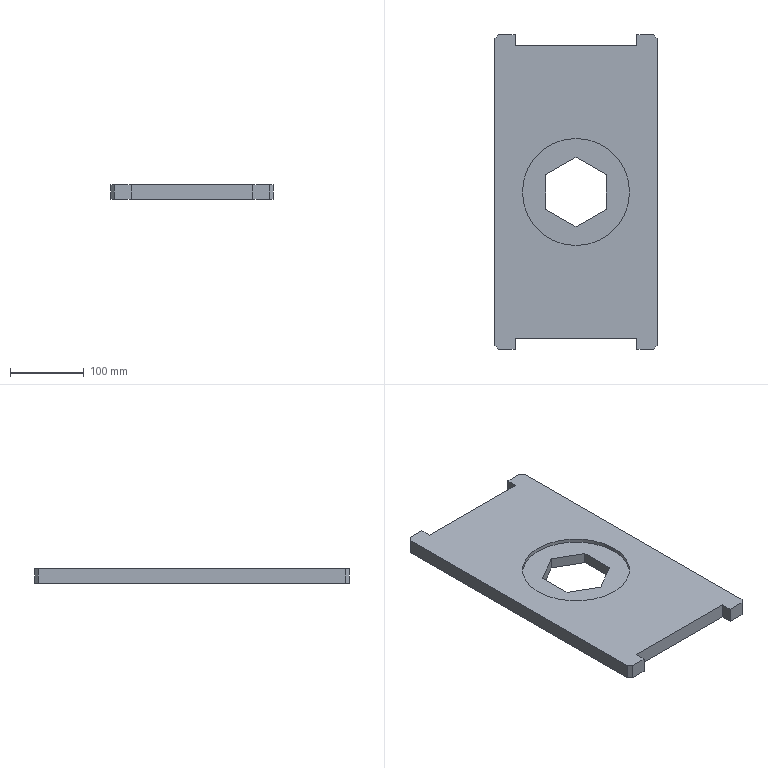Part | NX | features BREP 1 | 1 solid | 27 faces | box 220 x 426 x 20 mm | volume 1605748 mm3 | plane 25 | cylinder 2 | commonest cylinder face diameters 145 x2
STEP:
#1=CARTESIAN_POINT('',(-72.5,0.,15.));
#2=VERTEX_POINT('',#1);
#3=CARTESIAN_POINT('',(72.5,0.,15.));
#4=VERTEX_POINT('',#3);
#5=CARTESIAN_POINT('',(0.,0.,15.));
#6=DIRECTION('',(0.,0.,1.));
#7=DIRECTION('',(1.,0.,0.));
#8=AXIS2_PLACEMENT_3D('',#5,#6,#7);
#9=CIRCLE('',#8,72.5);
#10=EDGE_CURVE('',#2,#4,#9,.T.);
#11=ORIENTED_EDGE('',*,*,#10,.F.);
#12=CARTESIAN_POINT('',(-72.5,0.,20.));
#13=VERTEX_POINT('',#12);
#14=CARTESIAN_POINT('',(-72.5,0.,15.));
#15=DIRECTION('',(0.,0.,1.));
#16=VECTOR('',#15,1000.);
#17=LINE('',#14,#16);
#18=EDGE_CURVE('',#2,#13,#17,.T.);
#19=ORIENTED_EDGE('',*,*,#18,.T.);
#20=CARTESIAN_POINT('',(72.5,0.,20.));
#21=VERTEX_POINT('',#20);
#22=CARTESIAN_POINT('',(0.,0.,20.));
#23=DIRECTION('',(0.,0.,1.));
#24=DIRECTION('',(1.,0.,0.));
#25=AXIS2_PLACEMENT_3D('',#22,#23,#24);
#26=CIRCLE('',#25,72.5);
#27=EDGE_CURVE('',#13,#21,#26,.T.);
#28=ORIENTED_EDGE('',*,*,#27,.T.);
#29=CARTESIAN_POINT('',(72.5,0.,15.));
#30=DIRECTION('',(0.,0.,1.));
#31=VECTOR('',#30,1000.);
#32=LINE('',#29,#31);
#33=EDGE_CURVE('',#4,#21,#32,.T.);
#34=ORIENTED_EDGE('',*,*,#33,.F.);
#35=EDGE_LOOP('',(#11,#19,#28,#34));
#36=FACE_BOUND('',#35,.T.);
#37=CARTESIAN_POINT('',(0.,0.,15.));
#38=DIRECTION('',(0.,0.,1.));
#39=DIRECTION('',(-1.,0.,0.));
#40=AXIS2_PLACEMENT_3D('',#37,#38,#39);
#41=CYLINDRICAL_SURFACE('',#40,72.5);
#42=ADVANCED_FACE('',(#36),#41,.F.);
#43=CARTESIAN_POINT('',(40.703,23.5,15.));
#44=VERTEX_POINT('',#43);
#45=CARTESIAN_POINT('',(40.703,23.5,0.));
#46=VERTEX_POINT('',#45);
#47=CARTESIAN_POINT('',(40.703,23.5,20.));
#48=DIRECTION('',(0.,0.,-1.));
#49=VECTOR('',#48,1000.);
#50=LINE('',#47,#49);
#51=EDGE_CURVE('',#44,#46,#50,.T.);
#52=ORIENTED_EDGE('',*,*,#51,.F.);
#53=CARTESIAN_POINT('',(0.,47.,15.));
#54=VERTEX_POINT('',#53);
#55=CARTESIAN_POINT('',(40.703,23.5,15.));
#56=DIRECTION('',(-0.866,0.5,0.));
#57=VECTOR('',#56,1000.);
#58=LINE('',#55,#57);
#59=EDGE_CURVE('',#44,#54,#58,.T.);
#60=ORIENTED_EDGE('',*,*,#59,.T.);
#61=CARTESIAN_POINT('',(0.,47.,0.));
#62=VERTEX_POINT('',#61);
#63=CARTESIAN_POINT('',(0.,47.,20.));
#64=DIRECTION('',(0.,0.,-1.));
#65=VECTOR('',#64,1000.);
#66=LINE('',#63,#65);
#67=EDGE_CURVE('',#54,#62,#66,.T.);
#68=ORIENTED_EDGE('',*,*,#67,.T.);
#69=CARTESIAN_POINT('',(40.703,23.5,0.));
#70=DIRECTION('',(-0.866,0.5,0.));
#71=VECTOR('',#70,1000.);
#72=LINE('',#69,#71);
#73=EDGE_CURVE('',#46,#62,#72,.T.);
#74=ORIENTED_EDGE('',*,*,#73,.F.);
#75=EDGE_LOOP('',(#52,#60,#68,#74));
#76=FACE_BOUND('',#75,.T.);
#77=CARTESIAN_POINT('',(40.703,23.5,20.));
#78=DIRECTION('',(-0.5,-0.866,0.));
#79=DIRECTION('',(-0.866,0.5,0.));
#80=AXIS2_PLACEMENT_3D('',#77,#78,#79);
#81=PLANE('',#80);
#82=ADVANCED_FACE('',(#76),#81,.T.);
#83=ORIENTED_EDGE('',*,*,#67,.F.);
#84=CARTESIAN_POINT('',(-40.703,23.5,15.));
#85=VERTEX_POINT('',#84);
#86=CARTESIAN_POINT('',(0.,47.,15.));
#87=DIRECTION('',(-0.866,-0.5,0.));
#88=VECTOR('',#87,1000.);
#89=LINE('',#86,#88);
#90=EDGE_CURVE('',#54,#85,#89,.T.);
#91=ORIENTED_EDGE('',*,*,#90,.T.);
#92=CARTESIAN_POINT('',(-40.703,23.5,0.));
#93=VERTEX_POINT('',#92);
#94=CARTESIAN_POINT('',(-40.703,23.5,20.));
#95=DIRECTION('',(0.,0.,-1.));
#96=VECTOR('',#95,1000.);
#97=LINE('',#94,#96);
#98=EDGE_CURVE('',#85,#93,#97,.T.);
#99=ORIENTED_EDGE('',*,*,#98,.T.);
#100=CARTESIAN_POINT('',(0.,47.,0.));
#101=DIRECTION('',(-0.866,-0.5,0.));
#102=VECTOR('',#101,1000.);
#103=LINE('',#100,#102);
#104=EDGE_CURVE('',#62,#93,#103,.T.);
#105=ORIENTED_EDGE('',*,*,#104,.F.);
#106=EDGE_LOOP('',(#83,#91,#99,#105));
#107=FACE_BOUND('',#106,.T.);
#108=CARTESIAN_POINT('',(0.,47.,20.));
#109=DIRECTION('',(0.5,-0.866,0.));
#110=DIRECTION('',(-0.866,-0.5,0.));
#111=AXIS2_PLACEMENT_3D('',#108,#109,#110);
#112=PLANE('',#111);
#113=ADVANCED_FACE('',(#107),#112,.T.);
#114=ORIENTED_EDGE('',*,*,#98,.F.);
#115=CARTESIAN_POINT('',(-40.703,-23.5,15.));
#116=VERTEX_POINT('',#115);
#117=CARTESIAN_POINT('',(-40.703,23.5,15.));
#118=DIRECTION('',(0.,-1.,0.));
#119=VECTOR('',#118,1000.);
#120=LINE('',#117,#119);
#121=EDGE_CURVE('',#85,#116,#120,.T.);
#122=ORIENTED_EDGE('',*,*,#121,.T.);
#123=CARTESIAN_POINT('',(-40.703,-23.5,0.));
#124=VERTEX_POINT('',#123);
#125=CARTESIAN_POINT('',(-40.703,-23.5,20.));
#126=DIRECTION('',(0.,0.,-1.));
#127=VECTOR('',#126,1000.);
#128=LINE('',#125,#127);
#129=EDGE_CURVE('',#116,#124,#128,.T.);
#130=ORIENTED_EDGE('',*,*,#129,.T.);
#131=CARTESIAN_POINT('',(-40.703,23.5,0.));
#132=DIRECTION('',(0.,-1.,0.));
#133=VECTOR('',#132,1000.);
#134=LINE('',#131,#133);
#135=EDGE_CURVE('',#93,#124,#134,.T.);
#136=ORIENTED_EDGE('',*,*,#135,.F.);
#137=EDGE_LOOP('',(#114,#122,#130,#136));
#138=FACE_BOUND('',#137,.T.);
#139=CARTESIAN_POINT('',(-40.703,23.5,20.));
#140=DIRECTION('',(1.,0.,0.));
#141=DIRECTION('',(0.,-1.,0.));
#142=AXIS2_PLACEMENT_3D('',#139,#140,#141);
#143=PLANE('',#142);
#144=ADVANCED_FACE('',(#138),#143,.T.);
#145=ORIENTED_EDGE('',*,*,#129,.F.);
#146=CARTESIAN_POINT('',(0.,-47.,15.));
#147=VERTEX_POINT('',#146);
#148=CARTESIAN_POINT('',(-40.703,-23.5,15.));
#149=DIRECTION('',(0.866,-0.5,0.));
#150=VECTOR('',#149,1000.);
#151=LINE('',#148,#150);
#152=EDGE_CURVE('',#116,#147,#151,.T.);
#153=ORIENTED_EDGE('',*,*,#152,.T.);
#154=CARTESIAN_POINT('',(0.,-47.,0.));
#155=VERTEX_POINT('',#154);
#156=CARTESIAN_POINT('',(0.,-47.,20.));
#157=DIRECTION('',(0.,0.,-1.));
#158=VECTOR('',#157,1000.);
#159=LINE('',#156,#158);
#160=EDGE_CURVE('',#147,#155,#159,.T.);
#161=ORIENTED_EDGE('',*,*,#160,.T.);
#162=CARTESIAN_POINT('',(-40.703,-23.5,0.));
#163=DIRECTION('',(0.866,-0.5,0.));
#164=VECTOR('',#163,1000.);
#165=LINE('',#162,#164);
#166=EDGE_CURVE('',#124,#155,#165,.T.);
#167=ORIENTED_EDGE('',*,*,#166,.F.);
#168=EDGE_LOOP('',(#145,#153,#161,#167));
#169=FACE_BOUND('',#168,.T.);
#170=CARTESIAN_POINT('',(-40.703,-23.5,20.));
#171=DIRECTION('',(0.5,0.866,0.));
#172=DIRECTION('',(0.866,-0.5,0.));
#173=AXIS2_PLACEMENT_3D('',#170,#171,#172);
#174=PLANE('',#173);
#175=ADVANCED_FACE('',(#169),#174,.T.);
#176=ORIENTED_EDGE('',*,*,#160,.F.);
#177=CARTESIAN_POINT('',(40.703,-23.5,15.));
#178=VERTEX_POINT('',#177);
#179=CARTESIAN_POINT('',(0.,-47.,15.));
#180=DIRECTION('',(0.866,0.5,0.));
#181=VECTOR('',#180,1000.);
#182=LINE('',#179,#181);
#183=EDGE_CURVE('',#147,#178,#182,.T.);
#184=ORIENTED_EDGE('',*,*,#183,.T.);
#185=CARTESIAN_POINT('',(40.703,-23.5,0.));
#186=VERTEX_POINT('',#185);
#187=CARTESIAN_POINT('',(40.703,-23.5,20.));
#188=DIRECTION('',(0.,0.,-1.));
#189=VECTOR('',#188,1000.);
#190=LINE('',#187,#189);
#191=EDGE_CURVE('',#178,#186,#190,.T.);
#192=ORIENTED_EDGE('',*,*,#191,.T.);
#193=CARTESIAN_POINT('',(0.,-47.,0.));
#194=DIRECTION('',(0.866,0.5,0.));
#195=VECTOR('',#194,1000.);
#196=LINE('',#193,#195);
#197=EDGE_CURVE('',#155,#186,#196,.T.);
#198=ORIENTED_EDGE('',*,*,#197,.F.);
#199=EDGE_LOOP('',(#176,#184,#192,#198));
#200=FACE_BOUND('',#199,.T.);
#201=CARTESIAN_POINT('',(0.,-47.,20.));
#202=DIRECTION('',(-0.5,0.866,0.));
#203=DIRECTION('',(0.866,0.5,0.));
#204=AXIS2_PLACEMENT_3D('',#201,#202,#203);
#205=PLANE('',#204);
#206=ADVANCED_FACE('',(#200),#205,.T.);
#207=ORIENTED_EDGE('',*,*,#191,.F.);
#208=CARTESIAN_POINT('',(40.703,-23.5,15.));
#209=DIRECTION('',(0.,1.,0.));
#210=VECTOR('',#209,1000.);
#211=LINE('',#208,#210);
#212=EDGE_CURVE('',#178,#44,#211,.T.);
#213=ORIENTED_EDGE('',*,*,#212,.T.);
#214=ORIENTED_EDGE('',*,*,#51,.T.);
#215=CARTESIAN_POINT('',(40.703,-23.5,0.));
#216=DIRECTION('',(0.,1.,0.));
#217=VECTOR('',#216,1000.);
#218=LINE('',#215,#217);
#219=EDGE_CURVE('',#186,#46,#218,.T.);
#220=ORIENTED_EDGE('',*,*,#219,.F.);
#221=EDGE_LOOP('',(#207,#213,#214,#220));
#222=FACE_BOUND('',#221,.T.);
#223=CARTESIAN_POINT('',(40.703,-23.5,20.));
#224=DIRECTION('',(-1.,0.,0.));
#225=DIRECTION('',(0.,1.,0.));
#226=AXIS2_PLACEMENT_3D('',#223,#224,#225);
#227=PLANE('',#226);
#228=ADVANCED_FACE('',(#222),#227,.T.);
#229=CARTESIAN_POINT('',(0.,0.,20.));
#230=DIRECTION('',(0.,0.,1.));
#231=DIRECTION('',(1.,0.,0.));
#232=AXIS2_PLACEMENT_3D('',#229,#230,#231);
#233=CIRCLE('',#232,72.5);
#234=EDGE_CURVE('',#21,#13,#233,.T.);
#235=ORIENTED_EDGE('',*,*,#234,.F.);
#236=ORIENTED_EDGE('',*,*,#27,.F.);
#237=EDGE_LOOP('',(#235,#236));
#238=FACE_BOUND('',#237,.T.);
#239=CARTESIAN_POINT('',(-110.,208.,20.));
#240=VERTEX_POINT('',#239);
#241=CARTESIAN_POINT('',(-110.,-208.,20.));
#242=VERTEX_POINT('',#241);
#243=CARTESIAN_POINT('',(-110.,213.,20.));
#244=DIRECTION('',(0.,-1.,0.));
#245=VECTOR('',#244,1000.);
#246=LINE('',#243,#245);
#247=EDGE_CURVE('',#240,#242,#246,.T.);
#248=ORIENTED_EDGE('',*,*,#247,.T.);
#249=CARTESIAN_POINT('',(-105.,-213.,20.));
#250=VERTEX_POINT('',#249);
#251=CARTESIAN_POINT('',(-320.5,2.5,20.));
#252=DIRECTION('',(0.7071,-0.7071,0.));
#253=VECTOR('',#252,1000.);
#254=LINE('',#251,#253);
#255=EDGE_CURVE('',#242,#250,#254,.T.);
#256=ORIENTED_EDGE('',*,*,#255,.T.);
#257=CARTESIAN_POINT('',(-82.5,-213.,20.));
#258=VERTEX_POINT('',#257);
#259=CARTESIAN_POINT('',(-110.,-213.,20.));
#260=DIRECTION('',(1.,0.,0.));
#261=VECTOR('',#260,1000.);
#262=LINE('',#259,#261);
#263=EDGE_CURVE('',#250,#258,#262,.T.);
#264=ORIENTED_EDGE('',*,*,#263,.T.);
#265=CARTESIAN_POINT('',(-82.5,-198.,20.));
#266=VERTEX_POINT('',#265);
#267=CARTESIAN_POINT('',(-82.5,-198.,20.));
#268=DIRECTION('',(0.,1.,0.));
#269=VECTOR('',#268,1000.);
#270=LINE('',#267,#269);
#271=EDGE_CURVE('',#258,#266,#270,.T.);
#272=ORIENTED_EDGE('',*,*,#271,.T.);
#273=CARTESIAN_POINT('',(82.5,-198.,20.));
#274=VERTEX_POINT('',#273);
#275=CARTESIAN_POINT('',(82.5,-198.,20.));
#276=DIRECTION('',(1.,0.,0.));
#277=VECTOR('',#276,1000.);
#278=LINE('',#275,#277);
#279=EDGE_CURVE('',#266,#274,#278,.T.);
#280=ORIENTED_EDGE('',*,*,#279,.T.);
#281=CARTESIAN_POINT('',(82.5,-213.,20.));
#282=VERTEX_POINT('',#281);
#283=CARTESIAN_POINT('',(82.5,-198.,20.));
#284=DIRECTION('',(0.,-1.,0.));
#285=VECTOR('',#284,1000.);
#286=LINE('',#283,#285);
#287=EDGE_CURVE('',#274,#282,#286,.T.);
#288=ORIENTED_EDGE('',*,*,#287,.T.);
#289=CARTESIAN_POINT('',(105.,-213.,20.));
#290=VERTEX_POINT('',#289);
#291=CARTESIAN_POINT('',(82.5,-213.,20.));
#292=DIRECTION('',(1.,0.,0.));
#293=VECTOR('',#292,1000.);
#294=LINE('',#291,#293);
#295=EDGE_CURVE('',#282,#290,#294,.T.);
#296=ORIENTED_EDGE('',*,*,#295,.T.);
#297=CARTESIAN_POINT('',(110.,-208.,20.));
#298=VERTEX_POINT('',#297);
#299=CARTESIAN_POINT('',(210.5,-107.5,20.));
#300=DIRECTION('',(0.7071,0.7071,0.));
#301=VECTOR('',#300,1000.);
#302=LINE('',#299,#301);
#303=EDGE_CURVE('',#290,#298,#302,.T.);
#304=ORIENTED_EDGE('',*,*,#303,.T.);
#305=CARTESIAN_POINT('',(110.,208.,20.));
#306=VERTEX_POINT('',#305);
#307=CARTESIAN_POINT('',(110.,213.,20.));
#308=DIRECTION('',(0.,1.,0.));
#309=VECTOR('',#308,1000.);
#310=LINE('',#307,#309);
#311=EDGE_CURVE('',#298,#306,#310,.T.);
#312=ORIENTED_EDGE('',*,*,#311,.T.);
#313=CARTESIAN_POINT('',(105.,213.,20.));
#314=VERTEX_POINT('',#313);
#315=CARTESIAN_POINT('',(-2.5,320.5,20.));
#316=DIRECTION('',(-0.7071,0.7071,0.));
#317=VECTOR('',#316,1000.);
#318=LINE('',#315,#317);
#319=EDGE_CURVE('',#306,#314,#318,.T.);
#320=ORIENTED_EDGE('',*,*,#319,.T.);
#321=CARTESIAN_POINT('',(82.5,213.,20.));
#322=VERTEX_POINT('',#321);
#323=CARTESIAN_POINT('',(82.5,213.,20.));
#324=DIRECTION('',(-1.,0.,0.));
#325=VECTOR('',#324,1000.);
#326=LINE('',#323,#325);
#327=EDGE_CURVE('',#314,#322,#326,.T.);
#328=ORIENTED_EDGE('',*,*,#327,.T.);
#329=CARTESIAN_POINT('',(82.5,198.,20.));
#330=VERTEX_POINT('',#329);
#331=CARTESIAN_POINT('',(82.5,198.,20.));
#332=DIRECTION('',(0.,-1.,0.));
#333=VECTOR('',#332,1000.);
#334=LINE('',#331,#333);
#335=EDGE_CURVE('',#322,#330,#334,.T.);
#336=ORIENTED_EDGE('',*,*,#335,.T.);
#337=CARTESIAN_POINT('',(-82.5,198.,20.));
#338=VERTEX_POINT('',#337);
#339=CARTESIAN_POINT('',(82.5,198.,20.));
#340=DIRECTION('',(-1.,0.,0.));
#341=VECTOR('',#340,1000.);
#342=LINE('',#339,#341);
#343=EDGE_CURVE('',#330,#338,#342,.T.);
#344=ORIENTED_EDGE('',*,*,#343,.T.);
#345=CARTESIAN_POINT('',(-82.5,213.,20.));
#346=VERTEX_POINT('',#345);
#347=CARTESIAN_POINT('',(-82.5,198.,20.));
#348=DIRECTION('',(0.,1.,0.));
#349=VECTOR('',#348,1000.);
#350=LINE('',#347,#349);
#351=EDGE_CURVE('',#338,#346,#350,.T.);
#352=ORIENTED_EDGE('',*,*,#351,.T.);
#353=CARTESIAN_POINT('',(-105.,213.,20.));
#354=VERTEX_POINT('',#353);
#355=CARTESIAN_POINT('',(-110.,213.,20.));
#356=DIRECTION('',(-1.,0.,0.));
#357=VECTOR('',#356,1000.);
#358=LINE('',#355,#357);
#359=EDGE_CURVE('',#346,#354,#358,.T.);
#360=ORIENTED_EDGE('',*,*,#359,.T.);
#361=CARTESIAN_POINT('',(-107.5,210.5,20.));
#362=DIRECTION('',(-0.7071,-0.7071,0.));
#363=VECTOR('',#362,1000.);
#364=LINE('',#361,#363);
#365=EDGE_CURVE('',#354,#240,#364,.T.);
#366=ORIENTED_EDGE('',*,*,#365,.T.);
#367=EDGE_LOOP('',(#248,#256,#264,#272,#280,#288,#296,#304,#312,#320,#328,#336,#344,#352,#360,#366));
#368=FACE_BOUND('',#367,.T.);
#369=CARTESIAN_POINT('',(-110.,213.,20.));
#370=DIRECTION('',(0.,0.,1.));
#371=DIRECTION('',(-1.,0.,0.));
#372=AXIS2_PLACEMENT_3D('',#369,#370,#371);
#373=PLANE('',#372);
#374=ADVANCED_FACE('',(#238,#368),#373,.T.);
#375=CARTESIAN_POINT('',(-105.,-213.,0.));
#376=VERTEX_POINT('',#375);
#377=CARTESIAN_POINT('',(-82.5,-213.,0.));
#378=VERTEX_POINT('',#377);
#379=CARTESIAN_POINT('',(-110.,-213.,0.));
#380=DIRECTION('',(1.,0.,0.));
#381=VECTOR('',#380,1000.);
#382=LINE('',#379,#381);
#383=EDGE_CURVE('',#376,#378,#382,.T.);
#384=ORIENTED_EDGE('',*,*,#383,.F.);
#385=CARTESIAN_POINT('',(-110.,-208.,0.));
#386=VERTEX_POINT('',#385);
#387=CARTESIAN_POINT('',(-105.,-213.,0.));
#388=DIRECTION('',(-0.7071,0.7071,0.));
#389=VECTOR('',#388,1000.);
#390=LINE('',#387,#389);
#391=EDGE_CURVE('',#376,#386,#390,.T.);
#392=ORIENTED_EDGE('',*,*,#391,.T.);
#393=CARTESIAN_POINT('',(-110.,208.,0.));
#394=VERTEX_POINT('',#393);
#395=CARTESIAN_POINT('',(-110.,213.,0.));
#396=DIRECTION('',(0.,-1.,0.));
#397=VECTOR('',#396,1000.);
#398=LINE('',#395,#397);
#399=EDGE_CURVE('',#394,#386,#398,.T.);
#400=ORIENTED_EDGE('',*,*,#399,.F.);
#401=CARTESIAN_POINT('',(-105.,213.,0.));
#402=VERTEX_POINT('',#401);
#403=CARTESIAN_POINT('',(-110.,208.,0.));
#404=DIRECTION('',(0.7071,0.7071,0.));
#405=VECTOR('',#404,1000.);
#406=LINE('',#403,#405);
#407=EDGE_CURVE('',#394,#402,#406,.T.);
#408=ORIENTED_EDGE('',*,*,#407,.T.);
#409=CARTESIAN_POINT('',(-82.5,213.,0.));
#410=VERTEX_POINT('',#409);
#411=CARTESIAN_POINT('',(-110.,213.,0.));
#412=DIRECTION('',(-1.,0.,0.));
#413=VECTOR('',#412,1000.);
#414=LINE('',#411,#413);
#415=EDGE_CURVE('',#410,#402,#414,.T.);
#416=ORIENTED_EDGE('',*,*,#415,.F.);
#417=CARTESIAN_POINT('',(-82.5,198.,0.));
#418=VERTEX_POINT('',#417);
#419=CARTESIAN_POINT('',(-82.5,198.,0.));
#420=DIRECTION('',(0.,1.,0.));
#421=VECTOR('',#420,1000.);
#422=LINE('',#419,#421);
#423=EDGE_CURVE('',#418,#410,#422,.T.);
#424=ORIENTED_EDGE('',*,*,#423,.F.);
#425=CARTESIAN_POINT('',(82.5,198.,0.));
#426=VERTEX_POINT('',#425);
#427=CARTESIAN_POINT('',(82.5,198.,0.));
#428=DIRECTION('',(-1.,0.,0.));
#429=VECTOR('',#428,1000.);
#430=LINE('',#427,#429);
#431=EDGE_CURVE('',#426,#418,#430,.T.);
#432=ORIENTED_EDGE('',*,*,#431,.F.);
#433=CARTESIAN_POINT('',(82.5,213.,0.));
#434=VERTEX_POINT('',#433);
#435=CARTESIAN_POINT('',(82.5,198.,0.));
#436=DIRECTION('',(0.,-1.,0.));
#437=VECTOR('',#436,1000.);
#438=LINE('',#435,#437);
#439=EDGE_CURVE('',#434,#426,#438,.T.);
#440=ORIENTED_EDGE('',*,*,#439,.F.);
#441=CARTESIAN_POINT('',(105.,213.,0.));
#442=VERTEX_POINT('',#441);
#443=CARTESIAN_POINT('',(82.5,213.,0.));
#444=DIRECTION('',(-1.,0.,0.));
#445=VECTOR('',#444,1000.);
#446=LINE('',#443,#445);
#447=EDGE_CURVE('',#442,#434,#446,.T.);
#448=ORIENTED_EDGE('',*,*,#447,.F.);
#449=CARTESIAN_POINT('',(110.,208.,0.));
#450=VERTEX_POINT('',#449);
#451=CARTESIAN_POINT('',(105.,213.,0.));
#452=DIRECTION('',(0.7071,-0.7071,0.));
#453=VECTOR('',#452,1000.);
#454=LINE('',#451,#453);
#455=EDGE_CURVE('',#442,#450,#454,.T.);
#456=ORIENTED_EDGE('',*,*,#455,.T.);
#457=CARTESIAN_POINT('',(110.,-208.,0.));
#458=VERTEX_POINT('',#457);
#459=CARTESIAN_POINT('',(110.,213.,0.));
#460=DIRECTION('',(0.,1.,0.));
#461=VECTOR('',#460,1000.);
#462=LINE('',#459,#461);
#463=EDGE_CURVE('',#458,#450,#462,.T.);
#464=ORIENTED_EDGE('',*,*,#463,.F.);
#465=CARTESIAN_POINT('',(105.,-213.,0.));
#466=VERTEX_POINT('',#465);
#467=CARTESIAN_POINT('',(110.,-208.,0.));
#468=DIRECTION('',(-0.7071,-0.7071,0.));
#469=VECTOR('',#468,1000.);
#470=LINE('',#467,#469);
#471=EDGE_CURVE('',#458,#466,#470,.T.);
#472=ORIENTED_EDGE('',*,*,#471,.T.);
#473=CARTESIAN_POINT('',(82.5,-213.,0.));
#474=VERTEX_POINT('',#473);
#475=CARTESIAN_POINT('',(82.5,-213.,0.));
#476=DIRECTION('',(1.,0.,0.));
#477=VECTOR('',#476,1000.);
#478=LINE('',#475,#477);
#479=EDGE_CURVE('',#474,#466,#478,.T.);
#480=ORIENTED_EDGE('',*,*,#479,.F.);
#481=CARTESIAN_POINT('',(82.5,-198.,0.));
#482=VERTEX_POINT('',#481);
#483=CARTESIAN_POINT('',(82.5,-198.,0.));
#484=DIRECTION('',(0.,-1.,0.));
#485=VECTOR('',#484,1000.);
#486=LINE('',#483,#485);
#487=EDGE_CURVE('',#482,#474,#486,.T.);
#488=ORIENTED_EDGE('',*,*,#487,.F.);
#489=CARTESIAN_POINT('',(-82.5,-198.,0.));
#490=VERTEX_POINT('',#489);
#491=CARTESIAN_POINT('',(82.5,-198.,0.));
#492=DIRECTION('',(1.,0.,0.));
#493=VECTOR('',#492,1000.);
#494=LINE('',#491,#493);
#495=EDGE_CURVE('',#490,#482,#494,.T.);
#496=ORIENTED_EDGE('',*,*,#495,.F.);
#497=CARTESIAN_POINT('',(-82.5,-198.,0.));
#498=DIRECTION('',(0.,1.,0.));
#499=VECTOR('',#498,1000.);
#500=LINE('',#497,#499);
#501=EDGE_CURVE('',#378,#490,#500,.T.);
#502=ORIENTED_EDGE('',*,*,#501,.F.);
#503=EDGE_LOOP('',(#384,#392,#400,#408,#416,#424,#432,#440,#448,#456,#464,#472,#480,#488,#496,#502));
#504=FACE_BOUND('',#503,.T.);
#505=ORIENTED_EDGE('',*,*,#73,.T.);
#506=ORIENTED_EDGE('',*,*,#104,.T.);
#507=ORIENTED_EDGE('',*,*,#135,.T.);
#508=ORIENTED_EDGE('',*,*,#166,.T.);
#509=ORIENTED_EDGE('',*,*,#197,.T.);
#510=ORIENTED_EDGE('',*,*,#219,.T.);
#511=EDGE_LOOP('',(#505,#506,#507,#508,#509,#510));
#512=FACE_BOUND('',#511,.T.);
#513=CARTESIAN_POINT('',(-110.,213.,0.));
#514=DIRECTION('',(0.,0.,1.));
#515=DIRECTION('',(-1.,0.,0.));
#516=AXIS2_PLACEMENT_3D('',#513,#514,#515);
#517=PLANE('',#516);
#518=ADVANCED_FACE('',(#504,#512),#517,.F.);
#519=ORIENTED_EDGE('',*,*,#399,.T.);
#520=CARTESIAN_POINT('',(-110.,-208.,20.));
#521=DIRECTION('',(0.,0.,1.));
#522=VECTOR('',#521,1000.);
#523=LINE('',#520,#522);
#524=EDGE_CURVE('',#386,#242,#523,.T.);
#525=ORIENTED_EDGE('',*,*,#524,.T.);
#526=ORIENTED_EDGE('',*,*,#247,.F.);
#527=CARTESIAN_POINT('',(-110.,208.,20.));
#528=DIRECTION('',(0.,0.,-1.));
#529=VECTOR('',#528,1000.);
#530=LINE('',#527,#529);
#531=EDGE_CURVE('',#240,#394,#530,.T.);
#532=ORIENTED_EDGE('',*,*,#531,.T.);
#533=EDGE_LOOP('',(#519,#525,#526,#532));
#534=FACE_BOUND('',#533,.T.);
#535=CARTESIAN_POINT('',(-110.,213.,20.));
#536=DIRECTION('',(1.,0.,0.));
#537=DIRECTION('',(0.,-1.,0.));
#538=AXIS2_PLACEMENT_3D('',#535,#536,#537);
#539=PLANE('',#538);
#540=ADVANCED_FACE('',(#534),#539,.F.);
#541=ORIENTED_EDGE('',*,*,#263,.F.);
#542=CARTESIAN_POINT('',(-105.,-213.,20.));
#543=DIRECTION('',(0.,0.,-1.));
#544=VECTOR('',#543,1000.);
#545=LINE('',#542,#544);
#546=EDGE_CURVE('',#250,#376,#545,.T.);
#547=ORIENTED_EDGE('',*,*,#546,.T.);
#548=ORIENTED_EDGE('',*,*,#383,.T.);
#549=CARTESIAN_POINT('',(-82.5,-213.,20.));
#550=DIRECTION('',(0.,0.,-1.));
#551=VECTOR('',#550,1000.);
#552=LINE('',#549,#551);
#553=EDGE_CURVE('',#258,#378,#552,.T.);
#554=ORIENTED_EDGE('',*,*,#553,.F.);
#555=EDGE_LOOP('',(#541,#547,#548,#554));
#556=FACE_BOUND('',#555,.T.);
#557=CARTESIAN_POINT('',(-110.,-213.,20.));
#558=DIRECTION('',(0.,1.,0.));
#559=DIRECTION('',(1.,0.,0.));
#560=AXIS2_PLACEMENT_3D('',#557,#558,#559);
#561=PLANE('',#560);
#562=ADVANCED_FACE('',(#556),#561,.F.);
#563=ORIENTED_EDGE('',*,*,#501,.T.);
#564=CARTESIAN_POINT('',(-82.5,-198.,20.));
#565=DIRECTION('',(0.,0.,-1.));
#566=VECTOR('',#565,1000.);
#567=LINE('',#564,#566);
#568=EDGE_CURVE('',#266,#490,#567,.T.);
#569=ORIENTED_EDGE('',*,*,#568,.F.);
#570=ORIENTED_EDGE('',*,*,#271,.F.);
#571=ORIENTED_EDGE('',*,*,#553,.T.);
#572=EDGE_LOOP('',(#563,#569,#570,#571));
#573=FACE_BOUND('',#572,.T.);
#574=CARTESIAN_POINT('',(-82.5,-198.,20.));
#575=DIRECTION('',(-1.,0.,0.));
#576=DIRECTION('',(0.,0.,-1.));
#577=AXIS2_PLACEMENT_3D('',#574,#575,#576);
#578=PLANE('',#577);
#579=ADVANCED_FACE('',(#573),#578,.F.);
#580=ORIENTED_EDGE('',*,*,#495,.T.);
#581=CARTESIAN_POINT('',(82.5,-198.,20.));
#582=DIRECTION('',(0.,0.,-1.));
#583=VECTOR('',#582,1000.);
#584=LINE('',#581,#583);
#585=EDGE_CURVE('',#274,#482,#584,.T.);
#586=ORIENTED_EDGE('',*,*,#585,.F.);
#587=ORIENTED_EDGE('',*,*,#279,.F.);
#588=ORIENTED_EDGE('',*,*,#568,.T.);
#589=EDGE_LOOP('',(#580,#586,#587,#588));
#590=FACE_BOUND('',#589,.T.);
#591=CARTESIAN_POINT('',(82.5,-198.,20.));
#592=DIRECTION('',(0.,1.,0.));
#593=DIRECTION('',(1.,0.,0.));
#594=AXIS2_PLACEMENT_3D('',#591,#592,#593);
#595=PLANE('',#594);
#596=ADVANCED_FACE('',(#590),#595,.F.);
#597=ORIENTED_EDGE('',*,*,#487,.T.);
#598=CARTESIAN_POINT('',(82.5,-213.,20.));
#599=DIRECTION('',(0.,0.,-1.));
#600=VECTOR('',#599,1000.);
#601=LINE('',#598,#600);
#602=EDGE_CURVE('',#282,#474,#601,.T.);
#603=ORIENTED_EDGE('',*,*,#602,.F.);
#604=ORIENTED_EDGE('',*,*,#287,.F.);
#605=ORIENTED_EDGE('',*,*,#585,.T.);
#606=EDGE_LOOP('',(#597,#603,#604,#605));
#607=FACE_BOUND('',#606,.T.);
#608=CARTESIAN_POINT('',(82.5,-198.,20.));
#609=DIRECTION('',(1.,0.,0.));
#610=DIRECTION('',(0.,0.,1.));
#611=AXIS2_PLACEMENT_3D('',#608,#609,#610);
#612=PLANE('',#611);
#613=ADVANCED_FACE('',(#607),#612,.F.);
#614=ORIENTED_EDGE('',*,*,#479,.T.);
#615=CARTESIAN_POINT('',(105.,-213.,20.));
#616=DIRECTION('',(0.,0.,1.));
#617=VECTOR('',#616,1000.);
#618=LINE('',#615,#617);
#619=EDGE_CURVE('',#466,#290,#618,.T.);
#620=ORIENTED_EDGE('',*,*,#619,.T.);
#621=ORIENTED_EDGE('',*,*,#295,.F.);
#622=ORIENTED_EDGE('',*,*,#602,.T.);
#623=EDGE_LOOP('',(#614,#620,#621,#622));
#624=FACE_BOUND('',#623,.T.);
#625=CARTESIAN_POINT('',(82.5,-213.,20.));
#626=DIRECTION('',(0.,1.,0.));
#627=DIRECTION('',(1.,0.,0.));
#628=AXIS2_PLACEMENT_3D('',#625,#626,#627);
#629=PLANE('',#628);
#630=ADVANCED_FACE('',(#624),#629,.F.);
#631=ORIENTED_EDGE('',*,*,#311,.F.);
#632=CARTESIAN_POINT('',(110.,-208.,20.));
#633=DIRECTION('',(0.,0.,-1.));
#634=VECTOR('',#633,1000.);
#635=LINE('',#632,#634);
#636=EDGE_CURVE('',#298,#458,#635,.T.);
#637=ORIENTED_EDGE('',*,*,#636,.T.);
#638=ORIENTED_EDGE('',*,*,#463,.T.);
#639=CARTESIAN_POINT('',(110.,208.,20.));
#640=DIRECTION('',(0.,0.,1.));
#641=VECTOR('',#640,1000.);
#642=LINE('',#639,#641);
#643=EDGE_CURVE('',#450,#306,#642,.T.);
#644=ORIENTED_EDGE('',*,*,#643,.T.);
#645=EDGE_LOOP('',(#631,#637,#638,#644));
#646=FACE_BOUND('',#645,.T.);
#647=CARTESIAN_POINT('',(110.,213.,20.));
#648=DIRECTION('',(-1.,0.,0.));
#649=DIRECTION('',(0.,1.,0.));
#650=AXIS2_PLACEMENT_3D('',#647,#648,#649);
#651=PLANE('',#650);
#652=ADVANCED_FACE('',(#646),#651,.F.);
#653=ORIENTED_EDGE('',*,*,#327,.F.);
#654=CARTESIAN_POINT('',(105.,213.,20.));
#655=DIRECTION('',(0.,0.,-1.));
#656=VECTOR('',#655,1000.);
#657=LINE('',#654,#656);
#658=EDGE_CURVE('',#314,#442,#657,.T.);
#659=ORIENTED_EDGE('',*,*,#658,.T.);
#660=ORIENTED_EDGE('',*,*,#447,.T.);
#661=CARTESIAN_POINT('',(82.5,213.,20.));
#662=DIRECTION('',(0.,0.,-1.));
#663=VECTOR('',#662,1000.);
#664=LINE('',#661,#663);
#665=EDGE_CURVE('',#322,#434,#664,.T.);
#666=ORIENTED_EDGE('',*,*,#665,.F.);
#667=EDGE_LOOP('',(#653,#659,#660,#666));
#668=FACE_BOUND('',#667,.T.);
#669=CARTESIAN_POINT('',(82.5,213.,20.));
#670=DIRECTION('',(0.,-1.,0.));
#671=DIRECTION('',(0.,0.,1.));
#672=AXIS2_PLACEMENT_3D('',#669,#670,#671);
#673=PLANE('',#672);
#674=ADVANCED_FACE('',(#668),#673,.F.);
#675=ORIENTED_EDGE('',*,*,#439,.T.);
#676=CARTESIAN_POINT('',(82.5,198.,20.));
#677=DIRECTION('',(0.,0.,-1.));
#678=VECTOR('',#677,1000.);
#679=LINE('',#676,#678);
#680=EDGE_CURVE('',#330,#426,#679,.T.);
#681=ORIENTED_EDGE('',*,*,#680,.F.);
#682=ORIENTED_EDGE('',*,*,#335,.F.);
#683=ORIENTED_EDGE('',*,*,#665,.T.);
#684=EDGE_LOOP('',(#675,#681,#682,#683));
#685=FACE_BOUND('',#684,.T.);
#686=CARTESIAN_POINT('',(82.5,198.,20.));
#687=DIRECTION('',(1.,0.,0.));
#688=DIRECTION('',(0.,0.,1.));
#689=AXIS2_PLACEMENT_3D('',#686,#687,#688);
#690=PLANE('',#689);
#691=ADVANCED_FACE('',(#685),#690,.F.);
#692=ORIENTED_EDGE('',*,*,#431,.T.);
#693=CARTESIAN_POINT('',(-82.5,198.,20.));
#694=DIRECTION('',(0.,0.,-1.));
#695=VECTOR('',#694,1000.);
#696=LINE('',#693,#695);
#697=EDGE_CURVE('',#338,#418,#696,.T.);
#698=ORIENTED_EDGE('',*,*,#697,.F.);
#699=ORIENTED_EDGE('',*,*,#343,.F.);
#700=ORIENTED_EDGE('',*,*,#680,.T.);
#701=EDGE_LOOP('',(#692,#698,#699,#700));
#702=FACE_BOUND('',#701,.T.);
#703=CARTESIAN_POINT('',(82.5,198.,20.));
#704=DIRECTION('',(0.,-1.,0.));
#705=DIRECTION('',(-1.,0.,0.));
#706=AXIS2_PLACEMENT_3D('',#703,#704,#705);
#707=PLANE('',#706);
#708=ADVANCED_FACE('',(#702),#707,.F.);
#709=ORIENTED_EDGE('',*,*,#423,.T.);
#710=CARTESIAN_POINT('',(-82.5,213.,20.));
#711=DIRECTION('',(0.,0.,-1.));
#712=VECTOR('',#711,1000.);
#713=LINE('',#710,#712);
#714=EDGE_CURVE('',#346,#410,#713,.T.);
#715=ORIENTED_EDGE('',*,*,#714,.F.);
#716=ORIENTED_EDGE('',*,*,#351,.F.);
#717=ORIENTED_EDGE('',*,*,#697,.T.);
#718=EDGE_LOOP('',(#709,#715,#716,#717));
#719=FACE_BOUND('',#718,.T.);
#720=CARTESIAN_POINT('',(-82.5,198.,20.));
#721=DIRECTION('',(-1.,0.,0.));
#722=DIRECTION('',(0.,0.,-1.));
#723=AXIS2_PLACEMENT_3D('',#720,#721,#722);
#724=PLANE('',#723);
#725=ADVANCED_FACE('',(#719),#724,.F.);
#726=ORIENTED_EDGE('',*,*,#415,.T.);
#727=CARTESIAN_POINT('',(-105.,213.,20.));
#728=DIRECTION('',(0.,0.,1.));
#729=VECTOR('',#728,1000.);
#730=LINE('',#727,#729);
#731=EDGE_CURVE('',#402,#354,#730,.T.);
#732=ORIENTED_EDGE('',*,*,#731,.T.);
#733=ORIENTED_EDGE('',*,*,#359,.F.);
#734=ORIENTED_EDGE('',*,*,#714,.T.);
#735=EDGE_LOOP('',(#726,#732,#733,#734));
#736=FACE_BOUND('',#735,.T.);
#737=CARTESIAN_POINT('',(-110.,213.,20.));
#738=DIRECTION('',(0.,-1.,0.));
#739=DIRECTION('',(0.,0.,1.));
#740=AXIS2_PLACEMENT_3D('',#737,#738,#739);
#741=PLANE('',#740);
#742=ADVANCED_FACE('',(#736),#741,.F.);
#743=ORIENTED_EDGE('',*,*,#255,.F.);
#744=ORIENTED_EDGE('',*,*,#524,.F.);
#745=ORIENTED_EDGE('',*,*,#391,.F.);
#746=ORIENTED_EDGE('',*,*,#546,.F.);
#747=EDGE_LOOP('',(#743,#744,#745,#746));
#748=FACE_BOUND('',#747,.T.);
#749=CARTESIAN_POINT('',(-105.,-213.,20.));
#750=DIRECTION('',(0.7071,0.7071,0.));
#751=DIRECTION('',(0.7071,-0.7071,0.));
#752=AXIS2_PLACEMENT_3D('',#749,#750,#751);
#753=PLANE('',#752);
#754=ADVANCED_FACE('',(#748),#753,.F.);
#755=ORIENTED_EDGE('',*,*,#303,.F.);
#756=ORIENTED_EDGE('',*,*,#619,.F.);
#757=ORIENTED_EDGE('',*,*,#471,.F.);
#758=ORIENTED_EDGE('',*,*,#636,.F.);
#759=EDGE_LOOP('',(#755,#756,#757,#758));
#760=FACE_BOUND('',#759,.T.);
#761=CARTESIAN_POINT('',(110.,-208.,20.));
#762=DIRECTION('',(-0.7071,0.7071,0.));
#763=DIRECTION('',(0.7071,0.7071,0.));
#764=AXIS2_PLACEMENT_3D('',#761,#762,#763);
#765=PLANE('',#764);
#766=ADVANCED_FACE('',(#760),#765,.F.);
#767=ORIENTED_EDGE('',*,*,#365,.F.);
#768=ORIENTED_EDGE('',*,*,#731,.F.);
#769=ORIENTED_EDGE('',*,*,#407,.F.);
#770=ORIENTED_EDGE('',*,*,#531,.F.);
#771=EDGE_LOOP('',(#767,#768,#769,#770));
#772=FACE_BOUND('',#771,.T.);
#773=CARTESIAN_POINT('',(-110.,208.,20.));
#774=DIRECTION('',(0.7071,-0.7071,0.));
#775=DIRECTION('',(-0.7071,-0.7071,0.));
#776=AXIS2_PLACEMENT_3D('',#773,#774,#775);
#777=PLANE('',#776);
#778=ADVANCED_FACE('',(#772),#777,.F.);
#779=ORIENTED_EDGE('',*,*,#319,.F.);
#780=ORIENTED_EDGE('',*,*,#643,.F.);
#781=ORIENTED_EDGE('',*,*,#455,.F.);
#782=ORIENTED_EDGE('',*,*,#658,.F.);
#783=EDGE_LOOP('',(#779,#780,#781,#782));
#784=FACE_BOUND('',#783,.T.);
#785=CARTESIAN_POINT('',(105.,213.,20.));
#786=DIRECTION('',(-0.7071,-0.7071,0.));
#787=DIRECTION('',(-0.7071,0.7071,0.));
#788=AXIS2_PLACEMENT_3D('',#785,#786,#787);
#789=PLANE('',#788);
#790=ADVANCED_FACE('',(#784),#789,.F.);
#791=ORIENTED_EDGE('',*,*,#18,.F.);
#792=CARTESIAN_POINT('',(0.,0.,15.));
#793=DIRECTION('',(0.,0.,1.));
#794=DIRECTION('',(1.,0.,0.));
#795=AXIS2_PLACEMENT_3D('',#792,#793,#794);
#796=CIRCLE('',#795,72.5);
#797=EDGE_CURVE('',#4,#2,#796,.T.);
#798=ORIENTED_EDGE('',*,*,#797,.F.);
#799=ORIENTED_EDGE('',*,*,#33,.T.);
#800=ORIENTED_EDGE('',*,*,#234,.T.);
#801=EDGE_LOOP('',(#791,#798,#799,#800));
#802=FACE_BOUND('',#801,.T.);
#803=CARTESIAN_POINT('',(0.,0.,15.));
#804=DIRECTION('',(0.,0.,1.));
#805=DIRECTION('',(-1.,0.,0.));
#806=AXIS2_PLACEMENT_3D('',#803,#804,#805);
#807=CYLINDRICAL_SURFACE('',#806,72.5);
#808=ADVANCED_FACE('',(#802),#807,.F.);
#809=ORIENTED_EDGE('',*,*,#212,.F.);
#810=ORIENTED_EDGE('',*,*,#183,.F.);
#811=ORIENTED_EDGE('',*,*,#152,.F.);
#812=ORIENTED_EDGE('',*,*,#121,.F.);
#813=ORIENTED_EDGE('',*,*,#90,.F.);
#814=ORIENTED_EDGE('',*,*,#59,.F.);
#815=EDGE_LOOP('',(#809,#810,#811,#812,#813,#814));
#816=FACE_BOUND('',#815,.T.);
#817=ORIENTED_EDGE('',*,*,#797,.T.);
#818=ORIENTED_EDGE('',*,*,#10,.T.);
#819=EDGE_LOOP('',(#817,#818));
#820=FACE_BOUND('',#819,.T.);
#821=CARTESIAN_POINT('',(0.,0.,15.));
#822=DIRECTION('',(0.,0.,1.));
#823=DIRECTION('',(-1.,0.,0.));
#824=AXIS2_PLACEMENT_3D('',#821,#822,#823);
#825=PLANE('',#824);
#826=ADVANCED_FACE('',(#816,#820),#825,.T.);
#827=CLOSED_SHELL('',(#42,#82,#113,#144,#175,#206,#228,#374,#518,#540,#562,#579,#596,#613,#630,#652,#674,#691,#708,#725,#742,#754,#766,#778,#790,#808,#826));
#828=MANIFOLD_SOLID_BREP('',#827);
#829=(LENGTH_UNIT()NAMED_UNIT(*)SI_UNIT(.MILLI.,.METRE.));
#830=UNCERTAINTY_MEASURE_WITH_UNIT(LENGTH_MEASURE(0.00001),#829,'','');
#831=(NAMED_UNIT(*)PLANE_ANGLE_UNIT()SI_UNIT($,.RADIAN.));
#832=(NAMED_UNIT(*)SI_UNIT($,.STERADIAN.)SOLID_ANGLE_UNIT());
#833=(GEOMETRIC_REPRESENTATION_CONTEXT(3)GLOBAL_UNCERTAINTY_ASSIGNED_CONTEXT((#830))GLOBAL_UNIT_ASSIGNED_CONTEXT((#829,#831,#832))REPRESENTATION_CONTEXT('',''));
#834=ADVANCED_BREP_SHAPE_REPRESENTATION('',(#828),#833);